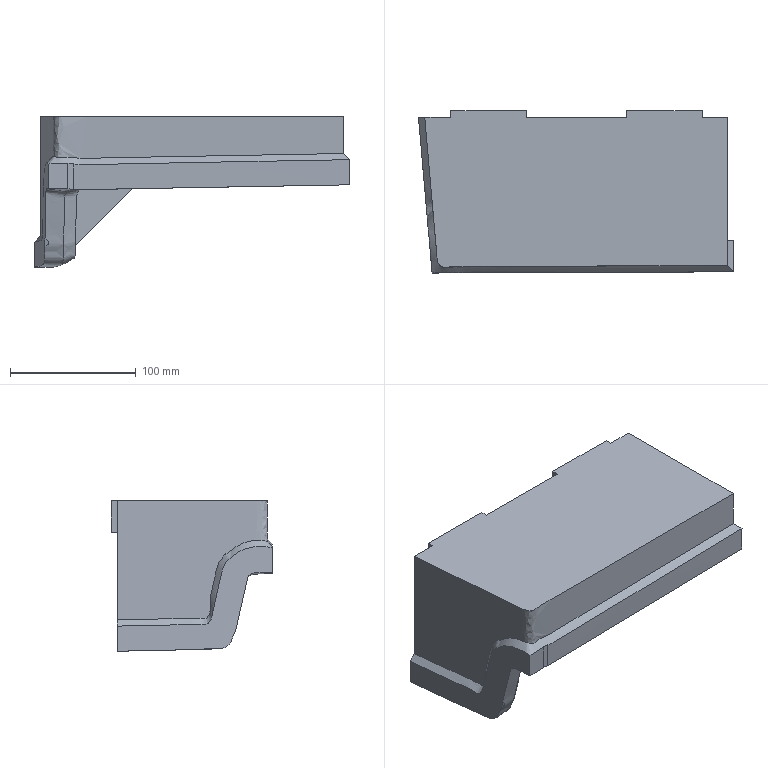Part | NX | features solid 2 | 1 solid | 36 faces | box 250.846 x 128.972 x 119.768 mm | volume 1145093 mm3 | plane 22 | spline 9 | cylinder 5 | commonest cylinder face diameters 30 x5